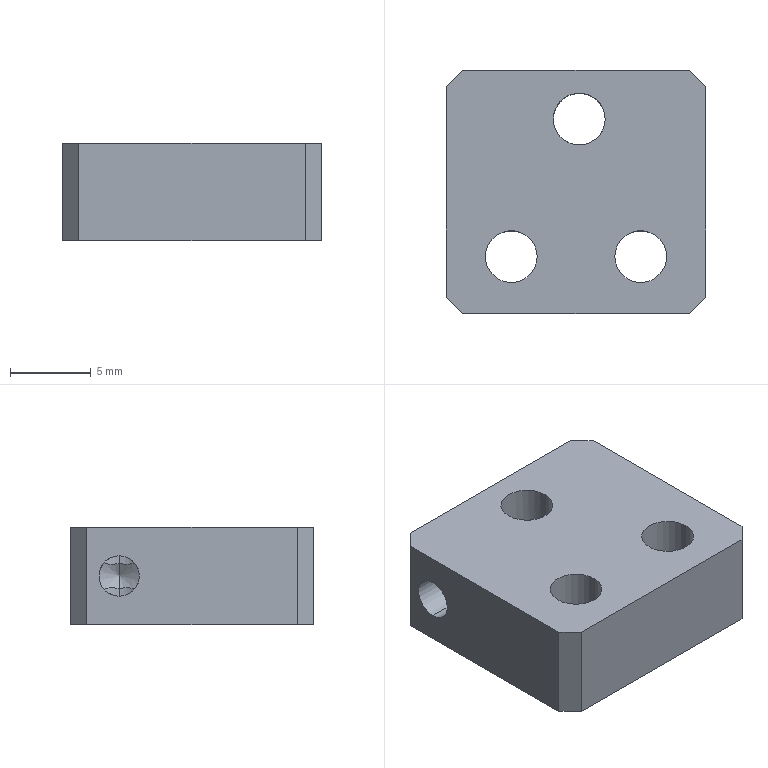Part | STEP file | 01-02-01 fibre mounting seat | 1 solid | 26 faces | box 16 x 15 x 6 mm | volume 1218 mm3 | cylinder 10 | plane 10 | cone 6 | commonest cylinder face diameters 3.2 x6 2.5 x4
STEP:
#1=CARTESIAN_POINT('',(-1.4,4.5,1.75));
#2=VERTEX_POINT('',#1);
#3=CARTESIAN_POINT('',(-1.4,4.5,4.25));
#4=VERTEX_POINT('',#3);
#5=CARTESIAN_POINT('',(-1.4,4.5,1.75));
#6=CARTESIAN_POINT('',(-1.4,4.414,1.75));
#7=CARTESIAN_POINT('',(-1.393,4.327,1.759));
#8=CARTESIAN_POINT('',(-1.366,4.16,1.794));
#9=CARTESIAN_POINT('',(-1.346,4.08,1.82));
#10=CARTESIAN_POINT('',(-1.271,3.851,1.919));
#11=CARTESIAN_POINT('',(-1.202,3.718,2.012));
#12=CARTESIAN_POINT('',(-1.056,3.5,2.234));
#13=CARTESIAN_POINT('',(-0.9765,3.412,2.365));
#14=CARTESIAN_POINT('',(-0.8475,3.287,2.658));
#15=CARTESIAN_POINT('',(-0.7986,3.25,2.829));
#16=CARTESIAN_POINT('',(-0.799,3.25,3.088));
#17=CARTESIAN_POINT('',(-0.8107,3.259,3.174));
#18=CARTESIAN_POINT('',(-0.8518,3.294,3.339));
#19=CARTESIAN_POINT('',(-0.8802,3.319,3.416));
#20=CARTESIAN_POINT('',(-0.9776,3.413,3.638));
#21=CARTESIAN_POINT('',(-1.056,3.5,3.766));
#22=CARTESIAN_POINT('',(-1.203,3.72,3.989));
#23=CARTESIAN_POINT('',(-1.271,3.85,4.08));
#24=CARTESIAN_POINT('',(-1.37,4.154,4.213));
#25=CARTESIAN_POINT('',(-1.4,4.326,4.25));
#26=CARTESIAN_POINT('',(-1.4,4.5,4.25));
#27=B_SPLINE_CURVE_WITH_KNOTS('',3,(#5,#6,#7,#8,#9,#10,#11,#12,#13,#14,#15,#16,#17,#18,#19,#20,#21,#22,#23,#24,#25,#26),.UNSPECIFIED.,.F.,.F.,(4,2,2,2,2,2,2,2,2,2,4),(0.004122,0.004379,0.004636,0.00515,0.005664,0.006178,0.006435,0.006692,0.007206,0.00772,0.008234),.UNSPECIFIED.);
#28=EDGE_CURVE('',#2,#4,#27,.T.);
#29=ORIENTED_EDGE('',*,*,#28,.F.);
#30=CARTESIAN_POINT('',(-8.,4.5,1.75));
#31=VERTEX_POINT('',#30);
#32=CARTESIAN_POINT('',(-8.,4.5,1.75));
#33=DIRECTION('',(-1.,0.,0.));
#34=VECTOR('',#33,1000.);
#35=LINE('',#32,#34);
#36=EDGE_CURVE('',#2,#31,#35,.T.);
#37=ORIENTED_EDGE('',*,*,#36,.T.);
#38=CARTESIAN_POINT('',(-8.,4.5,4.25));
#39=VERTEX_POINT('',#38);
#40=CARTESIAN_POINT('',(-8.,4.5,3.));
#41=DIRECTION('',(-1.,0.,0.));
#42=DIRECTION('',(0.,0.,1.));
#43=AXIS2_PLACEMENT_3D('',#40,#41,#42);
#44=CIRCLE('',#43,1.25);
#45=EDGE_CURVE('',#31,#39,#44,.T.);
#46=ORIENTED_EDGE('',*,*,#45,.T.);
#47=CARTESIAN_POINT('',(-8.,4.5,4.25));
#48=DIRECTION('',(-1.,0.,0.));
#49=VECTOR('',#48,1000.);
#50=LINE('',#47,#49);
#51=EDGE_CURVE('',#4,#39,#50,.T.);
#52=ORIENTED_EDGE('',*,*,#51,.F.);
#53=EDGE_LOOP('',(#29,#37,#46,#52));
#54=FACE_OUTER_BOUND('',#53,.T.);
#55=CARTESIAN_POINT('',(-8.,4.5,3.));
#56=DIRECTION('',(-1.,0.,0.));
#57=DIRECTION('',(0.,0.,1.));
#58=AXIS2_PLACEMENT_3D('',#55,#56,#57);
#59=CYLINDRICAL_SURFACE('',#58,1.25);
#60=ADVANCED_FACE('',(#54),#59,.F.);
#61=CARTESIAN_POINT('',(2.251,4.5,3.));
#62=VERTEX_POINT('',#61);
#63=CARTESIAN_POINT('',(1.8,4.5,3.751));
#64=VERTEX_POINT('',#63);
#65=CARTESIAN_POINT('',(1.5,4.5,4.25));
#66=DIRECTION('',(-0.515,0.,0.8572));
#67=VECTOR('',#66,1000.);
#68=LINE('',#65,#67);
#69=EDGE_CURVE('',#62,#64,#68,.T.);
#70=ORIENTED_EDGE('',*,*,#69,.F.);
#71=CARTESIAN_POINT('',(1.8,4.5,2.249));
#72=VERTEX_POINT('',#71);
#73=CARTESIAN_POINT('',(1.5,4.5,1.75));
#74=DIRECTION('',(-0.515,0.,-0.8572));
#75=VECTOR('',#74,1000.);
#76=LINE('',#73,#75);
#77=EDGE_CURVE('',#62,#72,#76,.T.);
#78=ORIENTED_EDGE('',*,*,#77,.T.);
#79=CARTESIAN_POINT('',(1.5,3.567,2.168));
#80=VERTEX_POINT('',#79);
#81=CARTESIAN_POINT('',(1.5,3.567,2.168));
#82=CARTESIAN_POINT('',(1.543,3.628,2.208));
#83=CARTESIAN_POINT('',(1.586,3.696,2.237));
#84=CARTESIAN_POINT('',(1.662,3.844,2.269));
#85=CARTESIAN_POINT('',(1.694,3.923,2.272));
#86=CARTESIAN_POINT('',(1.747,4.083,2.269));
#87=CARTESIAN_POINT('',(1.767,4.165,2.262));
#88=CARTESIAN_POINT('',(1.793,4.331,2.253));
#89=CARTESIAN_POINT('',(1.8,4.415,2.249));
#90=CARTESIAN_POINT('',(1.8,4.5,2.249));
#91=B_SPLINE_CURVE_WITH_KNOTS('',3,(#81,#82,#83,#84,#85,#86,#87,#88,#89,#90),.UNSPECIFIED.,.F.,.F.,(4,2,2,2,4),(0.00005832,0.0003106,0.0005629,0.0008152,0.001067),.UNSPECIFIED.);
#92=EDGE_CURVE('',#80,#72,#91,.T.);
#93=ORIENTED_EDGE('',*,*,#92,.F.);
#94=CARTESIAN_POINT('',(1.5,3.567,3.832));
#95=VERTEX_POINT('',#94);
#96=CARTESIAN_POINT('',(1.5,4.5,3.));
#97=DIRECTION('',(-1.,0.,0.));
#98=DIRECTION('',(0.,0.,1.));
#99=AXIS2_PLACEMENT_3D('',#96,#97,#98);
#100=CIRCLE('',#99,1.25);
#101=EDGE_CURVE('',#80,#95,#100,.T.);
#102=ORIENTED_EDGE('',*,*,#101,.T.);
#103=CARTESIAN_POINT('',(1.8,4.5,3.751));
#104=CARTESIAN_POINT('',(1.8,4.415,3.751));
#105=CARTESIAN_POINT('',(1.793,4.331,3.748));
#106=CARTESIAN_POINT('',(1.767,4.166,3.738));
#107=CARTESIAN_POINT('',(1.747,4.083,3.731));
#108=CARTESIAN_POINT('',(1.694,3.922,3.728));
#109=CARTESIAN_POINT('',(1.662,3.844,3.731));
#110=CARTESIAN_POINT('',(1.585,3.695,3.763));
#111=CARTESIAN_POINT('',(1.543,3.628,3.792));
#112=CARTESIAN_POINT('',(1.5,3.567,3.832));
#113=B_SPLINE_CURVE_WITH_KNOTS('',3,(#103,#104,#105,#106,#107,#108,#109,#110,#111,#112),.UNSPECIFIED.,.F.,.F.,(4,2,2,2,4),(0.001067,0.00132,0.001574,0.001827,0.00208),.UNSPECIFIED.);
#114=EDGE_CURVE('',#64,#95,#113,.T.);
#115=ORIENTED_EDGE('',*,*,#114,.F.);
#116=EDGE_LOOP('',(#70,#78,#93,#102,#115));
#117=FACE_OUTER_BOUND('',#116,.T.);
#118=CARTESIAN_POINT('',(1.5,4.5,3.));
#119=DIRECTION('',(-1.,0.,0.));
#120=DIRECTION('',(0.,0.,1.));
#121=AXIS2_PLACEMENT_3D('',#118,#119,#120);
#122=CONICAL_SURFACE('',#121,1.25,1.03);
#123=ADVANCED_FACE('',(#117),#122,.F.);
#124=CARTESIAN_POINT('',(5.6,-4.,1.55));
#125=VERTEX_POINT('',#124);
#126=CARTESIAN_POINT('',(2.4,-4.,1.55));
#127=VERTEX_POINT('',#126);
#128=CARTESIAN_POINT('',(4.,-4.,1.55));
#129=DIRECTION('',(0.,0.,-1.));
#130=DIRECTION('',(-1.,0.,0.));
#131=AXIS2_PLACEMENT_3D('',#128,#129,#130);
#132=CIRCLE('',#131,1.6);
#133=EDGE_CURVE('',#125,#127,#132,.T.);
#134=ORIENTED_EDGE('',*,*,#133,.F.);
#135=CARTESIAN_POINT('',(7.15,-4.,0.));
#136=VERTEX_POINT('',#135);
#137=CARTESIAN_POINT('',(7.15,-4.,0.));
#138=DIRECTION('',(0.7071,0.,-0.7071));
#139=VECTOR('',#138,1000.);
#140=LINE('',#137,#139);
#141=EDGE_CURVE('',#125,#136,#140,.T.);
#142=ORIENTED_EDGE('',*,*,#141,.T.);
#143=CARTESIAN_POINT('',(0.85,-4.,0.));
#144=VERTEX_POINT('',#143);
#145=CARTESIAN_POINT('',(4.,-4.,0.));
#146=DIRECTION('',(0.,0.,-1.));
#147=DIRECTION('',(-1.,0.,0.));
#148=AXIS2_PLACEMENT_3D('',#145,#146,#147);
#149=CIRCLE('',#148,3.15);
#150=EDGE_CURVE('',#136,#144,#149,.T.);
#151=ORIENTED_EDGE('',*,*,#150,.T.);
#152=CARTESIAN_POINT('',(0.85,-4.,0.));
#153=DIRECTION('',(-0.7071,0.,-0.7071));
#154=VECTOR('',#153,1000.);
#155=LINE('',#152,#154);
#156=EDGE_CURVE('',#127,#144,#155,.T.);
#157=ORIENTED_EDGE('',*,*,#156,.F.);
#158=EDGE_LOOP('',(#134,#142,#151,#157));
#159=FACE_OUTER_BOUND('',#158,.T.);
#160=CARTESIAN_POINT('',(4.,-4.,0.));
#161=DIRECTION('',(0.,0.,-1.));
#162=DIRECTION('',(-1.,0.,0.));
#163=AXIS2_PLACEMENT_3D('',#160,#161,#162);
#164=CONICAL_SURFACE('',#163,3.15,0.7854);
#165=ADVANCED_FACE('',(#159),#164,.F.);
#166=CARTESIAN_POINT('',(5.6,-4.,6.));
#167=VERTEX_POINT('',#166);
#168=CARTESIAN_POINT('',(2.4,-4.,6.));
#169=VERTEX_POINT('',#168);
#170=CARTESIAN_POINT('',(4.,-4.,6.));
#171=DIRECTION('',(0.,0.,-1.));
#172=DIRECTION('',(-1.,0.,0.));
#173=AXIS2_PLACEMENT_3D('',#170,#171,#172);
#174=CIRCLE('',#173,1.6);
#175=EDGE_CURVE('',#167,#169,#174,.T.);
#176=ORIENTED_EDGE('',*,*,#175,.F.);
#177=CARTESIAN_POINT('',(5.6,-4.,0.));
#178=DIRECTION('',(0.,0.,-1.));
#179=VECTOR('',#178,1000.);
#180=LINE('',#177,#179);
#181=EDGE_CURVE('',#167,#125,#180,.T.);
#182=ORIENTED_EDGE('',*,*,#181,.T.);
#183=ORIENTED_EDGE('',*,*,#133,.T.);
#184=CARTESIAN_POINT('',(2.4,-4.,0.));
#185=DIRECTION('',(0.,0.,-1.));
#186=VECTOR('',#185,1000.);
#187=LINE('',#184,#186);
#188=EDGE_CURVE('',#169,#127,#187,.T.);
#189=ORIENTED_EDGE('',*,*,#188,.F.);
#190=EDGE_LOOP('',(#176,#182,#183,#189));
#191=FACE_OUTER_BOUND('',#190,.T.);
#192=CARTESIAN_POINT('',(4.,-4.,0.));
#193=DIRECTION('',(0.,0.,-1.));
#194=DIRECTION('',(-1.,0.,0.));
#195=AXIS2_PLACEMENT_3D('',#192,#193,#194);
#196=CYLINDRICAL_SURFACE('',#195,1.6);
#197=ADVANCED_FACE('',(#191),#196,.F.);
#198=CARTESIAN_POINT('',(-2.4,-4.,1.55));
#199=VERTEX_POINT('',#198);
#200=CARTESIAN_POINT('',(-5.6,-4.,1.55));
#201=VERTEX_POINT('',#200);
#202=CARTESIAN_POINT('',(-4.,-4.,1.55));
#203=DIRECTION('',(0.,0.,-1.));
#204=DIRECTION('',(-1.,0.,0.));
#205=AXIS2_PLACEMENT_3D('',#202,#203,#204);
#206=CIRCLE('',#205,1.6);
#207=EDGE_CURVE('',#199,#201,#206,.T.);
#208=ORIENTED_EDGE('',*,*,#207,.F.);
#209=CARTESIAN_POINT('',(-0.85,-4.,0.));
#210=VERTEX_POINT('',#209);
#211=CARTESIAN_POINT('',(-0.85,-4.,0.));
#212=DIRECTION('',(0.7071,0.,-0.7071));
#213=VECTOR('',#212,1000.);
#214=LINE('',#211,#213);
#215=EDGE_CURVE('',#199,#210,#214,.T.);
#216=ORIENTED_EDGE('',*,*,#215,.T.);
#217=CARTESIAN_POINT('',(-7.15,-4.,0.));
#218=VERTEX_POINT('',#217);
#219=CARTESIAN_POINT('',(-4.,-4.,0.));
#220=DIRECTION('',(0.,0.,-1.));
#221=DIRECTION('',(-1.,0.,0.));
#222=AXIS2_PLACEMENT_3D('',#219,#220,#221);
#223=CIRCLE('',#222,3.15);
#224=EDGE_CURVE('',#210,#218,#223,.T.);
#225=ORIENTED_EDGE('',*,*,#224,.T.);
#226=CARTESIAN_POINT('',(-7.15,-4.,0.));
#227=DIRECTION('',(-0.7071,0.,-0.7071));
#228=VECTOR('',#227,1000.);
#229=LINE('',#226,#228);
#230=EDGE_CURVE('',#201,#218,#229,.T.);
#231=ORIENTED_EDGE('',*,*,#230,.F.);
#232=EDGE_LOOP('',(#208,#216,#225,#231));
#233=FACE_OUTER_BOUND('',#232,.T.);
#234=CARTESIAN_POINT('',(-4.,-4.,0.));
#235=DIRECTION('',(0.,0.,-1.));
#236=DIRECTION('',(-1.,0.,0.));
#237=AXIS2_PLACEMENT_3D('',#234,#235,#236);
#238=CONICAL_SURFACE('',#237,3.15,0.7854);
#239=ADVANCED_FACE('',(#233),#238,.F.);
#240=CARTESIAN_POINT('',(-2.4,-4.,6.));
#241=VERTEX_POINT('',#240);
#242=CARTESIAN_POINT('',(-5.6,-4.,6.));
#243=VERTEX_POINT('',#242);
#244=CARTESIAN_POINT('',(-4.,-4.,6.));
#245=DIRECTION('',(0.,0.,-1.));
#246=DIRECTION('',(-1.,0.,0.));
#247=AXIS2_PLACEMENT_3D('',#244,#245,#246);
#248=CIRCLE('',#247,1.6);
#249=EDGE_CURVE('',#241,#243,#248,.T.);
#250=ORIENTED_EDGE('',*,*,#249,.F.);
#251=CARTESIAN_POINT('',(-2.4,-4.,0.));
#252=DIRECTION('',(0.,0.,-1.));
#253=VECTOR('',#252,1000.);
#254=LINE('',#251,#253);
#255=EDGE_CURVE('',#241,#199,#254,.T.);
#256=ORIENTED_EDGE('',*,*,#255,.T.);
#257=ORIENTED_EDGE('',*,*,#207,.T.);
#258=CARTESIAN_POINT('',(-5.6,-4.,0.));
#259=DIRECTION('',(0.,0.,-1.));
#260=VECTOR('',#259,1000.);
#261=LINE('',#258,#260);
#262=EDGE_CURVE('',#243,#201,#261,.T.);
#263=ORIENTED_EDGE('',*,*,#262,.F.);
#264=EDGE_LOOP('',(#250,#256,#257,#263));
#265=FACE_OUTER_BOUND('',#264,.T.);
#266=CARTESIAN_POINT('',(-4.,-4.,0.));
#267=DIRECTION('',(0.,0.,-1.));
#268=DIRECTION('',(-1.,0.,0.));
#269=AXIS2_PLACEMENT_3D('',#266,#267,#268);
#270=CYLINDRICAL_SURFACE('',#269,1.6);
#271=ADVANCED_FACE('',(#265),#270,.F.);
#272=CARTESIAN_POINT('',(1.8,4.5,6.));
#273=VERTEX_POINT('',#272);
#274=CARTESIAN_POINT('',(-1.4,4.5,6.));
#275=VERTEX_POINT('',#274);
#276=CARTESIAN_POINT('',(0.1999,4.5,6.));
#277=DIRECTION('',(0.,0.,-1.));
#278=DIRECTION('',(-1.,0.,0.));
#279=AXIS2_PLACEMENT_3D('',#276,#277,#278);
#280=CIRCLE('',#279,1.6);
#281=EDGE_CURVE('',#273,#275,#280,.T.);
#282=ORIENTED_EDGE('',*,*,#281,.F.);
#283=CARTESIAN_POINT('',(1.8,4.5,6.));
#284=DIRECTION('',(0.,0.,-1.));
#285=VECTOR('',#284,1000.);
#286=LINE('',#283,#285);
#287=EDGE_CURVE('',#273,#64,#286,.T.);
#288=ORIENTED_EDGE('',*,*,#287,.T.);
#289=ORIENTED_EDGE('',*,*,#114,.T.);
#290=CARTESIAN_POINT('',(1.5,3.567,3.832));
#291=CARTESIAN_POINT('',(1.43,3.47,3.723));
#292=CARTESIAN_POINT('',(1.358,3.393,3.601));
#293=CARTESIAN_POINT('',(1.27,3.31,3.39));
#294=CARTESIAN_POINT('',(1.245,3.288,3.317));
#295=CARTESIAN_POINT('',(1.209,3.258,3.162));
#296=CARTESIAN_POINT('',(1.199,3.25,3.081));
#297=CARTESIAN_POINT('',(1.198,3.25,2.84));
#298=CARTESIAN_POINT('',(1.241,3.282,2.68));
#299=CARTESIAN_POINT('',(1.357,3.393,2.401));
#300=CARTESIAN_POINT('',(1.43,3.47,2.277));
#301=CARTESIAN_POINT('',(1.5,3.567,2.168));
#302=B_SPLINE_CURVE_WITH_KNOTS('',3,(#290,#291,#292,#293,#294,#295,#296,#297,#298,#299,#300,#301),.UNSPECIFIED.,.F.,.F.,(4,2,2,2,2,4),(0.,0.0004811,0.0007216,0.0009621,0.001443,0.001924),.UNSPECIFIED.);
#303=EDGE_CURVE('',#95,#80,#302,.T.);
#304=ORIENTED_EDGE('',*,*,#303,.T.);
#305=ORIENTED_EDGE('',*,*,#92,.T.);
#306=CARTESIAN_POINT('',(1.8,4.5,0.));
#307=VERTEX_POINT('',#306);
#308=CARTESIAN_POINT('',(1.8,4.5,6.));
#309=DIRECTION('',(0.,0.,-1.));
#310=VECTOR('',#309,1000.);
#311=LINE('',#308,#310);
#312=EDGE_CURVE('',#72,#307,#311,.T.);
#313=ORIENTED_EDGE('',*,*,#312,.T.);
#314=CARTESIAN_POINT('',(-1.4,4.5,0.));
#315=VERTEX_POINT('',#314);
#316=CARTESIAN_POINT('',(0.1999,4.5,0.));
#317=DIRECTION('',(0.,0.,-1.));
#318=DIRECTION('',(-1.,0.,0.));
#319=AXIS2_PLACEMENT_3D('',#316,#317,#318);
#320=CIRCLE('',#319,1.6);
#321=EDGE_CURVE('',#307,#315,#320,.T.);
#322=ORIENTED_EDGE('',*,*,#321,.T.);
#323=CARTESIAN_POINT('',(-1.4,4.5,6.));
#324=DIRECTION('',(0.,0.,-1.));
#325=VECTOR('',#324,1000.);
#326=LINE('',#323,#325);
#327=EDGE_CURVE('',#2,#315,#326,.T.);
#328=ORIENTED_EDGE('',*,*,#327,.F.);
#329=ORIENTED_EDGE('',*,*,#28,.T.);
#330=CARTESIAN_POINT('',(-1.4,4.5,6.));
#331=DIRECTION('',(0.,0.,-1.));
#332=VECTOR('',#331,1000.);
#333=LINE('',#330,#332);
#334=EDGE_CURVE('',#275,#4,#333,.T.);
#335=ORIENTED_EDGE('',*,*,#334,.F.);
#336=EDGE_LOOP('',(#282,#288,#289,#304,#305,#313,#322,#328,#329,#335));
#337=FACE_OUTER_BOUND('',#336,.T.);
#338=CARTESIAN_POINT('',(0.1999,4.5,6.));
#339=DIRECTION('',(0.,0.,-1.));
#340=DIRECTION('',(-1.,0.,0.));
#341=AXIS2_PLACEMENT_3D('',#338,#339,#340);
#342=CYLINDRICAL_SURFACE('',#341,1.6);
#343=ADVANCED_FACE('',(#337),#342,.F.);
#344=CARTESIAN_POINT('',(8.,-6.5,6.));
#345=VERTEX_POINT('',#344);
#346=CARTESIAN_POINT('',(8.,6.5,6.));
#347=VERTEX_POINT('',#346);
#348=CARTESIAN_POINT('',(8.,7.5,6.));
#349=DIRECTION('',(0.,1.,0.));
#350=VECTOR('',#349,1000.);
#351=LINE('',#348,#350);
#352=EDGE_CURVE('',#345,#347,#351,.T.);
#353=ORIENTED_EDGE('',*,*,#352,.F.);
#354=CARTESIAN_POINT('',(8.,-6.5,0.));
#355=VERTEX_POINT('',#354);
#356=CARTESIAN_POINT('',(8.,-6.5,6.));
#357=DIRECTION('',(0.,0.,-1.));
#358=VECTOR('',#357,1000.);
#359=LINE('',#356,#358);
#360=EDGE_CURVE('',#345,#355,#359,.T.);
#361=ORIENTED_EDGE('',*,*,#360,.T.);
#362=CARTESIAN_POINT('',(8.,6.5,0.));
#363=VERTEX_POINT('',#362);
#364=CARTESIAN_POINT('',(8.,7.5,0.));
#365=DIRECTION('',(0.,1.,0.));
#366=VECTOR('',#365,1000.);
#367=LINE('',#364,#366);
#368=EDGE_CURVE('',#355,#363,#367,.T.);
#369=ORIENTED_EDGE('',*,*,#368,.T.);
#370=CARTESIAN_POINT('',(8.,6.5,6.));
#371=DIRECTION('',(0.,0.,1.));
#372=VECTOR('',#371,1000.);
#373=LINE('',#370,#372);
#374=EDGE_CURVE('',#363,#347,#373,.T.);
#375=ORIENTED_EDGE('',*,*,#374,.T.);
#376=EDGE_LOOP('',(#353,#361,#369,#375));
#377=FACE_OUTER_BOUND('',#376,.T.);
#378=CARTESIAN_POINT('',(8.,7.5,6.));
#379=DIRECTION('',(-1.,0.,0.));
#380=DIRECTION('',(0.,-1.,0.));
#381=AXIS2_PLACEMENT_3D('',#378,#379,#380);
#382=PLANE('',#381);
#383=ADVANCED_FACE('',(#377),#382,.F.);
#384=CARTESIAN_POINT('',(7.,7.5,0.));
#385=VERTEX_POINT('',#384);
#386=CARTESIAN_POINT('',(-7.,7.5,0.));
#387=VERTEX_POINT('',#386);
#388=CARTESIAN_POINT('',(-8.,7.5,0.));
#389=DIRECTION('',(-1.,0.,0.));
#390=VECTOR('',#389,1000.);
#391=LINE('',#388,#390);
#392=EDGE_CURVE('',#385,#387,#391,.T.);
#393=ORIENTED_EDGE('',*,*,#392,.T.);
#394=CARTESIAN_POINT('',(-7.,7.5,6.));
#395=VERTEX_POINT('',#394);
#396=CARTESIAN_POINT('',(-7.,7.5,6.));
#397=DIRECTION('',(0.,0.,1.));
#398=VECTOR('',#397,1000.);
#399=LINE('',#396,#398);
#400=EDGE_CURVE('',#387,#395,#399,.T.);
#401=ORIENTED_EDGE('',*,*,#400,.T.);
#402=CARTESIAN_POINT('',(7.,7.5,6.));
#403=VERTEX_POINT('',#402);
#404=CARTESIAN_POINT('',(-8.,7.5,6.));
#405=DIRECTION('',(-1.,0.,0.));
#406=VECTOR('',#405,1000.);
#407=LINE('',#404,#406);
#408=EDGE_CURVE('',#403,#395,#407,.T.);
#409=ORIENTED_EDGE('',*,*,#408,.F.);
#410=CARTESIAN_POINT('',(7.,7.5,6.));
#411=DIRECTION('',(0.,0.,-1.));
#412=VECTOR('',#411,1000.);
#413=LINE('',#410,#412);
#414=EDGE_CURVE('',#403,#385,#413,.T.);
#415=ORIENTED_EDGE('',*,*,#414,.T.);
#416=EDGE_LOOP('',(#393,#401,#409,#415));
#417=FACE_OUTER_BOUND('',#416,.T.);
#418=CARTESIAN_POINT('',(-8.,7.5,6.));
#419=DIRECTION('',(0.,-1.,0.));
#420=DIRECTION('',(0.,0.,-1.));
#421=AXIS2_PLACEMENT_3D('',#418,#419,#420);
#422=PLANE('',#421);
#423=ADVANCED_FACE('',(#417),#422,.F.);
#424=CARTESIAN_POINT('',(-8.,4.5,3.));
#425=DIRECTION('',(-1.,0.,0.));
#426=DIRECTION('',(0.,0.,1.));
#427=AXIS2_PLACEMENT_3D('',#424,#425,#426);
#428=CIRCLE('',#427,1.25);
#429=EDGE_CURVE('',#39,#31,#428,.T.);
#430=ORIENTED_EDGE('',*,*,#429,.F.);
#431=ORIENTED_EDGE('',*,*,#45,.F.);
#432=EDGE_LOOP('',(#430,#431));
#433=FACE_BOUND('',#432,.T.);
#434=CARTESIAN_POINT('',(-8.,6.5,0.));
#435=VERTEX_POINT('',#434);
#436=CARTESIAN_POINT('',(-8.,-6.5,0.));
#437=VERTEX_POINT('',#436);
#438=CARTESIAN_POINT('',(-8.,7.5,0.));
#439=DIRECTION('',(0.,-1.,0.));
#440=VECTOR('',#439,1000.);
#441=LINE('',#438,#440);
#442=EDGE_CURVE('',#435,#437,#441,.T.);
#443=ORIENTED_EDGE('',*,*,#442,.T.);
#444=CARTESIAN_POINT('',(-8.,-6.5,6.));
#445=VERTEX_POINT('',#444);
#446=CARTESIAN_POINT('',(-8.,-6.5,6.));
#447=DIRECTION('',(0.,0.,1.));
#448=VECTOR('',#447,1000.);
#449=LINE('',#446,#448);
#450=EDGE_CURVE('',#437,#445,#449,.T.);
#451=ORIENTED_EDGE('',*,*,#450,.T.);
#452=CARTESIAN_POINT('',(-8.,6.5,6.));
#453=VERTEX_POINT('',#452);
#454=CARTESIAN_POINT('',(-8.,7.5,6.));
#455=DIRECTION('',(0.,-1.,0.));
#456=VECTOR('',#455,1000.);
#457=LINE('',#454,#456);
#458=EDGE_CURVE('',#453,#445,#457,.T.);
#459=ORIENTED_EDGE('',*,*,#458,.F.);
#460=CARTESIAN_POINT('',(-8.,6.5,6.));
#461=DIRECTION('',(0.,0.,-1.));
#462=VECTOR('',#461,1000.);
#463=LINE('',#460,#462);
#464=EDGE_CURVE('',#453,#435,#463,.T.);
#465=ORIENTED_EDGE('',*,*,#464,.T.);
#466=EDGE_LOOP('',(#443,#451,#459,#465));
#467=FACE_OUTER_BOUND('',#466,.T.);
#468=CARTESIAN_POINT('',(-8.,7.5,6.));
#469=DIRECTION('',(1.,0.,0.));
#470=DIRECTION('',(0.,1.,0.));
#471=AXIS2_PLACEMENT_3D('',#468,#469,#470);
#472=PLANE('',#471);
#473=ADVANCED_FACE('',(#433,#467),#472,.F.);
#474=CARTESIAN_POINT('',(-7.,-7.5,0.));
#475=VERTEX_POINT('',#474);
#476=CARTESIAN_POINT('',(7.,-7.5,0.));
#477=VERTEX_POINT('',#476);
#478=CARTESIAN_POINT('',(-8.,-7.5,0.));
#479=DIRECTION('',(1.,0.,0.));
#480=VECTOR('',#479,1000.);
#481=LINE('',#478,#480);
#482=EDGE_CURVE('',#475,#477,#481,.T.);
#483=ORIENTED_EDGE('',*,*,#482,.T.);
#484=CARTESIAN_POINT('',(7.,-7.5,6.));
#485=VERTEX_POINT('',#484);
#486=CARTESIAN_POINT('',(7.,-7.5,6.));
#487=DIRECTION('',(0.,0.,1.));
#488=VECTOR('',#487,1000.);
#489=LINE('',#486,#488);
#490=EDGE_CURVE('',#477,#485,#489,.T.);
#491=ORIENTED_EDGE('',*,*,#490,.T.);
#492=CARTESIAN_POINT('',(-7.,-7.5,6.));
#493=VERTEX_POINT('',#492);
#494=CARTESIAN_POINT('',(-8.,-7.5,6.));
#495=DIRECTION('',(1.,0.,0.));
#496=VECTOR('',#495,1000.);
#497=LINE('',#494,#496);
#498=EDGE_CURVE('',#493,#485,#497,.T.);
#499=ORIENTED_EDGE('',*,*,#498,.F.);
#500=CARTESIAN_POINT('',(-7.,-7.5,6.));
#501=DIRECTION('',(0.,0.,-1.));
#502=VECTOR('',#501,1000.);
#503=LINE('',#500,#502);
#504=EDGE_CURVE('',#493,#475,#503,.T.);
#505=ORIENTED_EDGE('',*,*,#504,.T.);
#506=EDGE_LOOP('',(#483,#491,#499,#505));
#507=FACE_OUTER_BOUND('',#506,.T.);
#508=CARTESIAN_POINT('',(-8.,-7.5,6.));
#509=DIRECTION('',(0.,1.,0.));
#510=DIRECTION('',(0.,0.,1.));
#511=AXIS2_PLACEMENT_3D('',#508,#509,#510);
#512=PLANE('',#511);
#513=ADVANCED_FACE('',(#507),#512,.F.);
#514=CARTESIAN_POINT('',(4.,-4.,6.));
#515=DIRECTION('',(0.,0.,-1.));
#516=DIRECTION('',(-1.,0.,0.));
#517=AXIS2_PLACEMENT_3D('',#514,#515,#516);
#518=CIRCLE('',#517,1.6);
#519=EDGE_CURVE('',#169,#167,#518,.T.);
#520=ORIENTED_EDGE('',*,*,#519,.T.);
#521=ORIENTED_EDGE('',*,*,#175,.T.);
#522=EDGE_LOOP('',(#520,#521));
#523=FACE_BOUND('',#522,.T.);
#524=CARTESIAN_POINT('',(-4.,-4.,6.));
#525=DIRECTION('',(0.,0.,-1.));
#526=DIRECTION('',(-1.,0.,0.));
#527=AXIS2_PLACEMENT_3D('',#524,#525,#526);
#528=CIRCLE('',#527,1.6);
#529=EDGE_CURVE('',#243,#241,#528,.T.);
#530=ORIENTED_EDGE('',*,*,#529,.T.);
#531=ORIENTED_EDGE('',*,*,#249,.T.);
#532=EDGE_LOOP('',(#530,#531));
#533=FACE_BOUND('',#532,.T.);
#534=CARTESIAN_POINT('',(0.1999,4.5,6.));
#535=DIRECTION('',(0.,0.,-1.));
#536=DIRECTION('',(-1.,0.,0.));
#537=AXIS2_PLACEMENT_3D('',#534,#535,#536);
#538=CIRCLE('',#537,1.6);
#539=EDGE_CURVE('',#275,#273,#538,.T.);
#540=ORIENTED_EDGE('',*,*,#539,.T.);
#541=ORIENTED_EDGE('',*,*,#281,.T.);
#542=EDGE_LOOP('',(#540,#541));
#543=FACE_BOUND('',#542,.T.);
#544=ORIENTED_EDGE('',*,*,#498,.T.);
#545=CARTESIAN_POINT('',(7.5,-7.,6.));
#546=DIRECTION('',(0.7071,0.7071,0.));
#547=VECTOR('',#546,1000.);
#548=LINE('',#545,#547);
#549=EDGE_CURVE('',#485,#345,#548,.T.);
#550=ORIENTED_EDGE('',*,*,#549,.T.);
#551=ORIENTED_EDGE('',*,*,#352,.T.);
#552=CARTESIAN_POINT('',(15.,-0.5,6.));
#553=DIRECTION('',(-0.7071,0.7071,0.));
#554=VECTOR('',#553,1000.);
#555=LINE('',#552,#554);
#556=EDGE_CURVE('',#347,#403,#555,.T.);
#557=ORIENTED_EDGE('',*,*,#556,.T.);
#558=ORIENTED_EDGE('',*,*,#408,.T.);
#559=CARTESIAN_POINT('',(-7.,7.5,6.));
#560=DIRECTION('',(-0.7071,-0.7071,0.));
#561=VECTOR('',#560,1000.);
#562=LINE('',#559,#561);
#563=EDGE_CURVE('',#395,#453,#562,.T.);
#564=ORIENTED_EDGE('',*,*,#563,.T.);
#565=ORIENTED_EDGE('',*,*,#458,.T.);
#566=CARTESIAN_POINT('',(0.5,-15.,6.));
#567=DIRECTION('',(0.7071,-0.7071,0.));
#568=VECTOR('',#567,1000.);
#569=LINE('',#566,#568);
#570=EDGE_CURVE('',#445,#493,#569,.T.);
#571=ORIENTED_EDGE('',*,*,#570,.T.);
#572=EDGE_LOOP('',(#544,#550,#551,#557,#558,#564,#565,#571));
#573=FACE_OUTER_BOUND('',#572,.T.);
#574=CARTESIAN_POINT('',(8.,-7.5,6.));
#575=DIRECTION('',(0.,0.,1.));
#576=DIRECTION('',(1.,0.,0.));
#577=AXIS2_PLACEMENT_3D('',#574,#575,#576);
#578=PLANE('',#577);
#579=ADVANCED_FACE('',(#523,#533,#543,#573),#578,.T.);
#580=CARTESIAN_POINT('',(4.,-4.,0.));
#581=DIRECTION('',(0.,0.,-1.));
#582=DIRECTION('',(-1.,0.,0.));
#583=AXIS2_PLACEMENT_3D('',#580,#581,#582);
#584=CIRCLE('',#583,3.15);
#585=EDGE_CURVE('',#144,#136,#584,.T.);
#586=ORIENTED_EDGE('',*,*,#585,.F.);
#587=ORIENTED_EDGE('',*,*,#150,.F.);
#588=EDGE_LOOP('',(#586,#587));
#589=FACE_BOUND('',#588,.T.);
#590=CARTESIAN_POINT('',(-4.,-4.,0.));
#591=DIRECTION('',(0.,0.,-1.));
#592=DIRECTION('',(-1.,0.,0.));
#593=AXIS2_PLACEMENT_3D('',#590,#591,#592);
#594=CIRCLE('',#593,3.15);
#595=EDGE_CURVE('',#218,#210,#594,.T.);
#596=ORIENTED_EDGE('',*,*,#595,.F.);
#597=ORIENTED_EDGE('',*,*,#224,.F.);
#598=EDGE_LOOP('',(#596,#597));
#599=FACE_BOUND('',#598,.T.);
#600=CARTESIAN_POINT('',(0.1999,4.5,0.));
#601=DIRECTION('',(0.,0.,-1.));
#602=DIRECTION('',(-1.,0.,0.));
#603=AXIS2_PLACEMENT_3D('',#600,#601,#602);
#604=CIRCLE('',#603,1.6);
#605=EDGE_CURVE('',#315,#307,#604,.T.);
#606=ORIENTED_EDGE('',*,*,#605,.F.);
#607=ORIENTED_EDGE('',*,*,#321,.F.);
#608=EDGE_LOOP('',(#606,#607));
#609=FACE_BOUND('',#608,.T.);
#610=ORIENTED_EDGE('',*,*,#368,.F.);
#611=CARTESIAN_POINT('',(8.,-6.5,0.));
#612=DIRECTION('',(-0.7071,-0.7071,0.));
#613=VECTOR('',#612,1000.);
#614=LINE('',#611,#613);
#615=EDGE_CURVE('',#355,#477,#614,.T.);
#616=ORIENTED_EDGE('',*,*,#615,.T.);
#617=ORIENTED_EDGE('',*,*,#482,.F.);
#618=CARTESIAN_POINT('',(-7.,-7.5,0.));
#619=DIRECTION('',(-0.7071,0.7071,0.));
#620=VECTOR('',#619,1000.);
#621=LINE('',#618,#620);
#622=EDGE_CURVE('',#475,#437,#621,.T.);
#623=ORIENTED_EDGE('',*,*,#622,.T.);
#624=ORIENTED_EDGE('',*,*,#442,.F.);
#625=CARTESIAN_POINT('',(-8.,6.5,0.));
#626=DIRECTION('',(0.7071,0.7071,0.));
#627=VECTOR('',#626,1000.);
#628=LINE('',#625,#627);
#629=EDGE_CURVE('',#435,#387,#628,.T.);
#630=ORIENTED_EDGE('',*,*,#629,.T.);
#631=ORIENTED_EDGE('',*,*,#392,.F.);
#632=CARTESIAN_POINT('',(7.,7.5,0.));
#633=DIRECTION('',(0.7071,-0.7071,0.));
#634=VECTOR('',#633,1000.);
#635=LINE('',#632,#634);
#636=EDGE_CURVE('',#385,#363,#635,.T.);
#637=ORIENTED_EDGE('',*,*,#636,.T.);
#638=EDGE_LOOP('',(#610,#616,#617,#623,#624,#630,#631,#637));
#639=FACE_OUTER_BOUND('',#638,.T.);
#640=CARTESIAN_POINT('',(8.,-7.5,0.));
#641=DIRECTION('',(0.,0.,1.));
#642=DIRECTION('',(1.,0.,0.));
#643=AXIS2_PLACEMENT_3D('',#640,#641,#642);
#644=PLANE('',#643);
#645=ADVANCED_FACE('',(#589,#599,#609,#639),#644,.F.);
#646=ORIENTED_EDGE('',*,*,#287,.F.);
#647=ORIENTED_EDGE('',*,*,#539,.F.);
#648=ORIENTED_EDGE('',*,*,#334,.T.);
#649=CARTESIAN_POINT('',(-1.4,4.5,4.25));
#650=CARTESIAN_POINT('',(-1.4,4.587,4.25));
#651=CARTESIAN_POINT('',(-1.393,4.673,4.241));
#652=CARTESIAN_POINT('',(-1.366,4.839,4.206));
#653=CARTESIAN_POINT('',(-1.346,4.921,4.18));
#654=CARTESIAN_POINT('',(-1.272,5.148,4.082));
#655=CARTESIAN_POINT('',(-1.203,5.281,3.988));
#656=CARTESIAN_POINT('',(-1.057,5.499,3.767));
#657=CARTESIAN_POINT('',(-0.9773,5.587,3.637));
#658=CARTESIAN_POINT('',(-0.8804,5.681,3.417));
#659=CARTESIAN_POINT('',(-0.8514,5.706,3.338));
#660=CARTESIAN_POINT('',(-0.8107,5.741,3.173));
#661=CARTESIAN_POINT('',(-0.7989,5.75,3.086));
#662=CARTESIAN_POINT('',(-0.7989,5.75,2.914));
#663=CARTESIAN_POINT('',(-0.8106,5.741,2.827));
#664=CARTESIAN_POINT('',(-0.8514,5.706,2.662));
#665=CARTESIAN_POINT('',(-0.8798,5.682,2.585));
#666=CARTESIAN_POINT('',(-0.9775,5.587,2.362));
#667=CARTESIAN_POINT('',(-1.056,5.501,2.235));
#668=CARTESIAN_POINT('',(-1.204,5.28,2.01));
#669=CARTESIAN_POINT('',(-1.271,5.151,1.92));
#670=CARTESIAN_POINT('',(-1.346,4.92,1.82));
#671=CARTESIAN_POINT('',(-1.366,4.84,1.794));
#672=CARTESIAN_POINT('',(-1.393,4.673,1.759));
#673=CARTESIAN_POINT('',(-1.4,4.586,1.75));
#674=CARTESIAN_POINT('',(-1.4,4.5,1.75));
#675=B_SPLINE_CURVE_WITH_KNOTS('',3,(#649,#650,#651,#652,#653,#654,#655,#656,#657,#658,#659,#660,#661,#662,#663,#664,#665,#666,#667,#668,#669,#670,#671,#672,#673,#674),.UNSPECIFIED.,.F.,.F.,(4,2,2,2,2,2,2,2,2,2,2,2,4),(0.,0.0002576,0.0005153,0.001031,0.001546,0.001803,0.002061,0.002319,0.002576,0.003092,0.003607,0.003864,0.004122),.UNSPECIFIED.);
#676=EDGE_CURVE('',#4,#2,#675,.T.);
#677=ORIENTED_EDGE('',*,*,#676,.T.);
#678=ORIENTED_EDGE('',*,*,#327,.T.);
#679=ORIENTED_EDGE('',*,*,#605,.T.);
#680=ORIENTED_EDGE('',*,*,#312,.F.);
#681=CARTESIAN_POINT('',(1.5,5.433,2.168));
#682=VERTEX_POINT('',#681);
#683=CARTESIAN_POINT('',(1.8,4.5,2.249));
#684=CARTESIAN_POINT('',(1.8,4.585,2.249));
#685=CARTESIAN_POINT('',(1.793,4.669,2.252));
#686=CARTESIAN_POINT('',(1.767,4.834,2.262));
#687=CARTESIAN_POINT('',(1.747,4.917,2.269));
#688=CARTESIAN_POINT('',(1.694,5.078,2.272));
#689=CARTESIAN_POINT('',(1.662,5.156,2.269));
#690=CARTESIAN_POINT('',(1.585,5.305,2.237));
#691=CARTESIAN_POINT('',(1.543,5.372,2.208));
#692=CARTESIAN_POINT('',(1.5,5.433,2.168));
#693=B_SPLINE_CURVE_WITH_KNOTS('',3,(#683,#684,#685,#686,#687,#688,#689,#690,#691,#692),.UNSPECIFIED.,.F.,.F.,(4,2,2,2,4),(0.001067,0.00132,0.001574,0.001827,0.00208),.UNSPECIFIED.);
#694=EDGE_CURVE('',#72,#682,#693,.T.);
#695=ORIENTED_EDGE('',*,*,#694,.T.);
#696=CARTESIAN_POINT('',(1.5,5.433,3.832));
#697=VERTEX_POINT('',#696);
#698=CARTESIAN_POINT('',(1.5,5.433,2.168));
#699=CARTESIAN_POINT('',(1.43,5.53,2.277));
#700=CARTESIAN_POINT('',(1.358,5.607,2.399));
#701=CARTESIAN_POINT('',(1.27,5.69,2.61));
#702=CARTESIAN_POINT('',(1.245,5.712,2.683));
#703=CARTESIAN_POINT('',(1.209,5.742,2.838));
#704=CARTESIAN_POINT('',(1.199,5.75,2.919));
#705=CARTESIAN_POINT('',(1.198,5.75,3.16));
#706=CARTESIAN_POINT('',(1.241,5.718,3.32));
#707=CARTESIAN_POINT('',(1.357,5.607,3.599));
#708=CARTESIAN_POINT('',(1.43,5.53,3.723));
#709=CARTESIAN_POINT('',(1.5,5.433,3.832));
#710=B_SPLINE_CURVE_WITH_KNOTS('',3,(#698,#699,#700,#701,#702,#703,#704,#705,#706,#707,#708,#709),.UNSPECIFIED.,.F.,.F.,(4,2,2,2,2,4),(0.,0.0004811,0.0007216,0.0009621,0.001443,0.001924),.UNSPECIFIED.);
#711=EDGE_CURVE('',#682,#697,#710,.T.);
#712=ORIENTED_EDGE('',*,*,#711,.T.);
#713=CARTESIAN_POINT('',(1.5,5.433,3.832));
#714=CARTESIAN_POINT('',(1.543,5.372,3.792));
#715=CARTESIAN_POINT('',(1.586,5.304,3.763));
#716=CARTESIAN_POINT('',(1.662,5.156,3.731));
#717=CARTESIAN_POINT('',(1.694,5.077,3.728));
#718=CARTESIAN_POINT('',(1.747,4.917,3.731));
#719=CARTESIAN_POINT('',(1.767,4.835,3.738));
#720=CARTESIAN_POINT('',(1.793,4.669,3.747));
#721=CARTESIAN_POINT('',(1.8,4.585,3.751));
#722=CARTESIAN_POINT('',(1.8,4.5,3.751));
#723=B_SPLINE_CURVE_WITH_KNOTS('',3,(#713,#714,#715,#716,#717,#718,#719,#720,#721,#722),.UNSPECIFIED.,.F.,.F.,(4,2,2,2,4),(0.00005832,0.0003106,0.0005629,0.0008152,0.001067),.UNSPECIFIED.);
#724=EDGE_CURVE('',#697,#64,#723,.T.);
#725=ORIENTED_EDGE('',*,*,#724,.T.);
#726=EDGE_LOOP('',(#646,#647,#648,#677,#678,#679,#680,#695,#712,#725));
#727=FACE_OUTER_BOUND('',#726,.T.);
#728=CARTESIAN_POINT('',(0.1999,4.5,6.));
#729=DIRECTION('',(0.,0.,-1.));
#730=DIRECTION('',(-1.,0.,0.));
#731=AXIS2_PLACEMENT_3D('',#728,#729,#730);
#732=CYLINDRICAL_SURFACE('',#731,1.6);
#733=ADVANCED_FACE('',(#727),#732,.F.);
#734=ORIENTED_EDGE('',*,*,#255,.F.);
#735=ORIENTED_EDGE('',*,*,#529,.F.);
#736=ORIENTED_EDGE('',*,*,#262,.T.);
#737=CARTESIAN_POINT('',(-4.,-4.,1.55));
#738=DIRECTION('',(0.,0.,-1.));
#739=DIRECTION('',(-1.,0.,0.));
#740=AXIS2_PLACEMENT_3D('',#737,#738,#739);
#741=CIRCLE('',#740,1.6);
#742=EDGE_CURVE('',#201,#199,#741,.T.);
#743=ORIENTED_EDGE('',*,*,#742,.T.);
#744=EDGE_LOOP('',(#734,#735,#736,#743));
#745=FACE_OUTER_BOUND('',#744,.T.);
#746=CARTESIAN_POINT('',(-4.,-4.,0.));
#747=DIRECTION('',(0.,0.,-1.));
#748=DIRECTION('',(-1.,0.,0.));
#749=AXIS2_PLACEMENT_3D('',#746,#747,#748);
#750=CYLINDRICAL_SURFACE('',#749,1.6);
#751=ADVANCED_FACE('',(#745),#750,.F.);
#752=ORIENTED_EDGE('',*,*,#215,.F.);
#753=ORIENTED_EDGE('',*,*,#742,.F.);
#754=ORIENTED_EDGE('',*,*,#230,.T.);
#755=ORIENTED_EDGE('',*,*,#595,.T.);
#756=EDGE_LOOP('',(#752,#753,#754,#755));
#757=FACE_OUTER_BOUND('',#756,.T.);
#758=CARTESIAN_POINT('',(-4.,-4.,0.));
#759=DIRECTION('',(0.,0.,-1.));
#760=DIRECTION('',(-1.,0.,0.));
#761=AXIS2_PLACEMENT_3D('',#758,#759,#760);
#762=CONICAL_SURFACE('',#761,3.15,0.7854);
#763=ADVANCED_FACE('',(#757),#762,.F.);
#764=ORIENTED_EDGE('',*,*,#181,.F.);
#765=ORIENTED_EDGE('',*,*,#519,.F.);
#766=ORIENTED_EDGE('',*,*,#188,.T.);
#767=CARTESIAN_POINT('',(4.,-4.,1.55));
#768=DIRECTION('',(0.,0.,-1.));
#769=DIRECTION('',(-1.,0.,0.));
#770=AXIS2_PLACEMENT_3D('',#767,#768,#769);
#771=CIRCLE('',#770,1.6);
#772=EDGE_CURVE('',#127,#125,#771,.T.);
#773=ORIENTED_EDGE('',*,*,#772,.T.);
#774=EDGE_LOOP('',(#764,#765,#766,#773));
#775=FACE_OUTER_BOUND('',#774,.T.);
#776=CARTESIAN_POINT('',(4.,-4.,0.));
#777=DIRECTION('',(0.,0.,-1.));
#778=DIRECTION('',(-1.,0.,0.));
#779=AXIS2_PLACEMENT_3D('',#776,#777,#778);
#780=CYLINDRICAL_SURFACE('',#779,1.6);
#781=ADVANCED_FACE('',(#775),#780,.F.);
#782=ORIENTED_EDGE('',*,*,#141,.F.);
#783=ORIENTED_EDGE('',*,*,#772,.F.);
#784=ORIENTED_EDGE('',*,*,#156,.T.);
#785=ORIENTED_EDGE('',*,*,#585,.T.);
#786=EDGE_LOOP('',(#782,#783,#784,#785));
#787=FACE_OUTER_BOUND('',#786,.T.);
#788=CARTESIAN_POINT('',(4.,-4.,0.));
#789=DIRECTION('',(0.,0.,-1.));
#790=DIRECTION('',(-1.,0.,0.));
#791=AXIS2_PLACEMENT_3D('',#788,#789,#790);
#792=CONICAL_SURFACE('',#791,3.15,0.7854);
#793=ADVANCED_FACE('',(#787),#792,.F.);
#794=ORIENTED_EDGE('',*,*,#77,.F.);
#795=ORIENTED_EDGE('',*,*,#69,.T.);
#796=ORIENTED_EDGE('',*,*,#724,.F.);
#797=CARTESIAN_POINT('',(1.5,4.5,3.));
#798=DIRECTION('',(-1.,0.,0.));
#799=DIRECTION('',(0.,0.,1.));
#800=AXIS2_PLACEMENT_3D('',#797,#798,#799);
#801=CIRCLE('',#800,1.25);
#802=EDGE_CURVE('',#697,#682,#801,.T.);
#803=ORIENTED_EDGE('',*,*,#802,.T.);
#804=ORIENTED_EDGE('',*,*,#694,.F.);
#805=EDGE_LOOP('',(#794,#795,#796,#803,#804));
#806=FACE_OUTER_BOUND('',#805,.T.);
#807=CARTESIAN_POINT('',(1.5,4.5,3.));
#808=DIRECTION('',(-1.,0.,0.));
#809=DIRECTION('',(0.,0.,1.));
#810=AXIS2_PLACEMENT_3D('',#807,#808,#809);
#811=CONICAL_SURFACE('',#810,1.25,1.03);
#812=ADVANCED_FACE('',(#806),#811,.F.);
#813=ORIENTED_EDGE('',*,*,#101,.F.);
#814=ORIENTED_EDGE('',*,*,#303,.F.);
#815=EDGE_LOOP('',(#813,#814));
#816=FACE_OUTER_BOUND('',#815,.T.);
#817=CARTESIAN_POINT('',(-8.,4.5,3.));
#818=DIRECTION('',(-1.,0.,0.));
#819=DIRECTION('',(0.,0.,1.));
#820=AXIS2_PLACEMENT_3D('',#817,#818,#819);
#821=CYLINDRICAL_SURFACE('',#820,1.25);
#822=ADVANCED_FACE('',(#816),#821,.F.);
#823=ORIENTED_EDGE('',*,*,#802,.F.);
#824=ORIENTED_EDGE('',*,*,#711,.F.);
#825=EDGE_LOOP('',(#823,#824));
#826=FACE_OUTER_BOUND('',#825,.T.);
#827=CARTESIAN_POINT('',(-8.,4.5,3.));
#828=DIRECTION('',(-1.,0.,0.));
#829=DIRECTION('',(0.,0.,1.));
#830=AXIS2_PLACEMENT_3D('',#827,#828,#829);
#831=CYLINDRICAL_SURFACE('',#830,1.25);
#832=ADVANCED_FACE('',(#826),#831,.F.);
#833=ORIENTED_EDGE('',*,*,#36,.F.);
#834=ORIENTED_EDGE('',*,*,#676,.F.);
#835=ORIENTED_EDGE('',*,*,#51,.T.);
#836=ORIENTED_EDGE('',*,*,#429,.T.);
#837=EDGE_LOOP('',(#833,#834,#835,#836));
#838=FACE_OUTER_BOUND('',#837,.T.);
#839=CARTESIAN_POINT('',(-8.,4.5,3.));
#840=DIRECTION('',(-1.,0.,0.));
#841=DIRECTION('',(0.,0.,1.));
#842=AXIS2_PLACEMENT_3D('',#839,#840,#841);
#843=CYLINDRICAL_SURFACE('',#842,1.25);
#844=ADVANCED_FACE('',(#838),#843,.F.);
#845=ORIENTED_EDGE('',*,*,#549,.F.);
#846=ORIENTED_EDGE('',*,*,#490,.F.);
#847=ORIENTED_EDGE('',*,*,#615,.F.);
#848=ORIENTED_EDGE('',*,*,#360,.F.);
#849=EDGE_LOOP('',(#845,#846,#847,#848));
#850=FACE_OUTER_BOUND('',#849,.T.);
#851=CARTESIAN_POINT('',(8.,-6.5,6.));
#852=DIRECTION('',(-0.7071,0.7071,0.));
#853=DIRECTION('',(-0.7071,-0.7071,0.));
#854=AXIS2_PLACEMENT_3D('',#851,#852,#853);
#855=PLANE('',#854);
#856=ADVANCED_FACE('',(#850),#855,.F.);
#857=ORIENTED_EDGE('',*,*,#570,.F.);
#858=ORIENTED_EDGE('',*,*,#450,.F.);
#859=ORIENTED_EDGE('',*,*,#622,.F.);
#860=ORIENTED_EDGE('',*,*,#504,.F.);
#861=EDGE_LOOP('',(#857,#858,#859,#860));
#862=FACE_OUTER_BOUND('',#861,.T.);
#863=CARTESIAN_POINT('',(-7.,-7.5,6.));
#864=DIRECTION('',(0.7071,0.7071,0.));
#865=DIRECTION('',(-0.7071,0.7071,0.));
#866=AXIS2_PLACEMENT_3D('',#863,#864,#865);
#867=PLANE('',#866);
#868=ADVANCED_FACE('',(#862),#867,.F.);
#869=ORIENTED_EDGE('',*,*,#563,.F.);
#870=ORIENTED_EDGE('',*,*,#400,.F.);
#871=ORIENTED_EDGE('',*,*,#629,.F.);
#872=ORIENTED_EDGE('',*,*,#464,.F.);
#873=EDGE_LOOP('',(#869,#870,#871,#872));
#874=FACE_OUTER_BOUND('',#873,.T.);
#875=CARTESIAN_POINT('',(-8.,6.5,6.));
#876=DIRECTION('',(0.7071,-0.7071,0.));
#877=DIRECTION('',(0.7071,0.7071,0.));
#878=AXIS2_PLACEMENT_3D('',#875,#876,#877);
#879=PLANE('',#878);
#880=ADVANCED_FACE('',(#874),#879,.F.);
#881=ORIENTED_EDGE('',*,*,#556,.F.);
#882=ORIENTED_EDGE('',*,*,#374,.F.);
#883=ORIENTED_EDGE('',*,*,#636,.F.);
#884=ORIENTED_EDGE('',*,*,#414,.F.);
#885=EDGE_LOOP('',(#881,#882,#883,#884));
#886=FACE_OUTER_BOUND('',#885,.T.);
#887=CARTESIAN_POINT('',(7.,7.5,6.));
#888=DIRECTION('',(-0.7071,-0.7071,0.));
#889=DIRECTION('',(0.7071,-0.7071,0.));
#890=AXIS2_PLACEMENT_3D('',#887,#888,#889);
#891=PLANE('',#890);
#892=ADVANCED_FACE('',(#886),#891,.F.);
#893=CLOSED_SHELL('',(#60,#123,#165,#197,#239,#271,#343,#383,#423,#473,#513,#579,#645,#733,#751,#763,#781,#793,#812,#822,#832,#844,#856,#868,#880,#892));
#894=MANIFOLD_SOLID_BREP('',#893);
#895=CARTESIAN_POINT('',(0.,0.,0.));
#896=DIRECTION('',(0.,0.,1.));
#897=DIRECTION('',(1.,0.,0.));
#898=AXIS2_PLACEMENT_3D('',#895,#896,#897);
#899=(LENGTH_UNIT()NAMED_UNIT(*)SI_UNIT(.MILLI.,.METRE.));
#900=UNCERTAINTY_MEASURE_WITH_UNIT(LENGTH_MEASURE(0.00001),#899,'','');
#901=(NAMED_UNIT(*)PLANE_ANGLE_UNIT()SI_UNIT($,.RADIAN.));
#902=(NAMED_UNIT(*)SI_UNIT($,.STERADIAN.)SOLID_ANGLE_UNIT());
#903=(GEOMETRIC_REPRESENTATION_CONTEXT(3)GLOBAL_UNCERTAINTY_ASSIGNED_CONTEXT((#900))GLOBAL_UNIT_ASSIGNED_CONTEXT((#899,#901,#902))REPRESENTATION_CONTEXT('',''));
#904=ADVANCED_BREP_SHAPE_REPRESENTATION('',(#894,#898),#903);